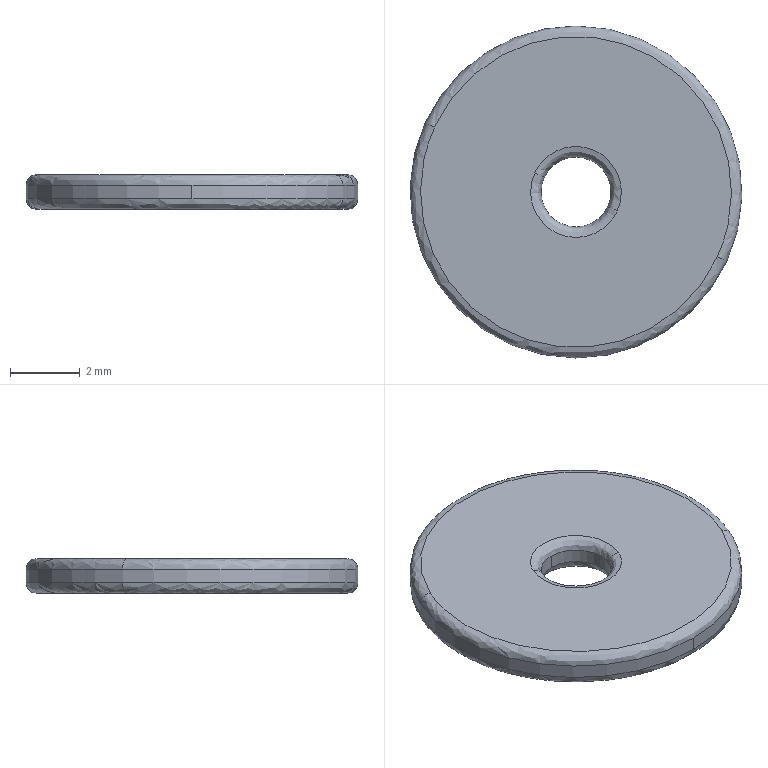Part | SolidWorks | features BaseBody 1 | 1 solid | 14 faces | box 9.5 x 9.5 x 1 mm | volume 66.343 mm3 | spline 8 | cylinder 4 | plane 2 | commonest cylinder face diameters 2 x2 9.5 x2
STEP:
#1=CARTESIAN_POINT('',(562.414,-175.786,282.579));
#2=VERTEX_POINT('',#1);
#3=CARTESIAN_POINT('',(554.328,-172.067,282.579));
#4=VERTEX_POINT('',#3);
#5=CARTESIAN_POINT('',(562.414,-175.786,282.579));
#6=CARTESIAN_POINT('',(558.694,-183.872,282.579));
#7=CARTESIAN_POINT('',(550.609,-180.152,282.579));
#8=CARTESIAN_POINT('',(554.328,-172.067,282.579));
#9=(BOUNDED_CURVE()B_SPLINE_CURVE(3,(#5,#6,#7,#8),.UNSPECIFIED.,.F.,.F.)B_SPLINE_CURVE_WITH_KNOTS((4,4),(0.,1.),.UNSPECIFIED.)CURVE()GEOMETRIC_REPRESENTATION_ITEM()RATIONAL_B_SPLINE_CURVE((1.,0.3333,0.3333,1.))REPRESENTATION_ITEM(''));
#10=EDGE_CURVE('',#2,#4,#9,.T.);
#11=ORIENTED_EDGE('',*,*,#10,.T.);
#12=CARTESIAN_POINT('',(554.056,-171.941,282.279));
#13=VERTEX_POINT('',#12);
#14=CARTESIAN_POINT('',(554.328,-172.067,282.279));
#15=DIRECTION('',(-0.4179,-0.9085,-0.000000003));
#16=DIRECTION('',(-0.9085,0.4179,0.000000002));
#17=AXIS2_PLACEMENT_3D('',#14,#15,#16);
#18=CIRCLE('',#17,0.3);
#19=EDGE_CURVE('',#4,#13,#18,.T.);
#20=ORIENTED_EDGE('',*,*,#19,.T.);
#21=CARTESIAN_POINT('',(558.371,-178.677,282.279));
#22=VERTEX_POINT('',#21);
#23=CARTESIAN_POINT('',(558.371,-173.927,282.279));
#24=DIRECTION('',(0.000000001,-0.000000003,1.));
#25=DIRECTION('',(0.9085,-0.4179,-0.000000002));
#26=AXIS2_PLACEMENT_3D('',#23,#24,#25);
#27=CIRCLE('',#26,4.75);
#28=EDGE_CURVE('',#13,#22,#27,.T.);
#29=ORIENTED_EDGE('',*,*,#28,.T.);
#30=CARTESIAN_POINT('',(562.686,-175.912,282.279));
#31=VERTEX_POINT('',#30);
#32=CARTESIAN_POINT('',(558.371,-173.927,282.279));
#33=DIRECTION('',(0.000000001,-0.000000003,1.));
#34=DIRECTION('',(0.9085,-0.4179,-0.000000002));
#35=AXIS2_PLACEMENT_3D('',#32,#33,#34);
#36=CIRCLE('',#35,4.75);
#37=EDGE_CURVE('',#22,#31,#36,.T.);
#38=ORIENTED_EDGE('',*,*,#37,.T.);
#39=CARTESIAN_POINT('',(562.414,-175.786,282.279));
#40=DIRECTION('',(0.4179,0.9085,0.000000003));
#41=DIRECTION('',(0.9085,-0.4179,-0.000000002));
#42=AXIS2_PLACEMENT_3D('',#39,#40,#41);
#43=CIRCLE('',#42,0.3);
#44=EDGE_CURVE('',#2,#31,#43,.T.);
#45=ORIENTED_EDGE('',*,*,#44,.F.);
#46=EDGE_LOOP('',(#11,#20,#29,#38,#45));
#47=FACE_OUTER_BOUND('',#46,.T.);
#48=CARTESIAN_POINT('',(554.328,-172.067,282.579));
#49=CARTESIAN_POINT('',(550.609,-180.152,282.579));
#50=CARTESIAN_POINT('',(558.694,-183.872,282.579));
#51=CARTESIAN_POINT('',(562.414,-175.786,282.579));
#52=CARTESIAN_POINT('',(554.169,-171.993,282.579));
#53=CARTESIAN_POINT('',(550.302,-180.398,282.579));
#54=CARTESIAN_POINT('',(558.707,-184.265,282.579));
#55=CARTESIAN_POINT('',(562.573,-175.86,282.579));
#56=CARTESIAN_POINT('',(554.056,-171.941,282.455));
#57=CARTESIAN_POINT('',(550.085,-180.572,282.455));
#58=CARTESIAN_POINT('',(558.716,-184.542,282.455));
#59=CARTESIAN_POINT('',(562.686,-175.912,282.455));
#60=CARTESIAN_POINT('',(554.056,-171.941,282.279));
#61=CARTESIAN_POINT('',(550.085,-180.572,282.279));
#62=CARTESIAN_POINT('',(558.716,-184.542,282.279));
#63=CARTESIAN_POINT('',(562.686,-175.912,282.279));
#64=(BOUNDED_SURFACE()B_SPLINE_SURFACE(3,3,((#48,#49,#50,#51),(#52,#53,#54,#55),(#56,#57,#58,#59),(#60,#61,#62,#63)),.UNSPECIFIED.,.F.,.F.,.T.)B_SPLINE_SURFACE_WITH_KNOTS((4,4),(4,4),(0.,1.),(0.,1.),.UNSPECIFIED.)GEOMETRIC_REPRESENTATION_ITEM()RATIONAL_B_SPLINE_SURFACE(((1.,0.3333,0.3333,1.),(0.8047,0.2682,0.2682,0.8047),(0.8047,0.2682,0.2682,0.8047),(1.,0.3333,0.3333,1.)))REPRESENTATION_ITEM('')SURFACE());
#65=ADVANCED_FACE('',(#47),#64,.T.);
#66=CARTESIAN_POINT('',(558.371,-174.927,282.279));
#67=VERTEX_POINT('',#66);
#68=CARTESIAN_POINT('',(557.463,-173.509,282.279));
#69=VERTEX_POINT('',#68);
#70=CARTESIAN_POINT('',(558.371,-173.927,282.279));
#71=DIRECTION('',(-0.000000001,0.000000003,-1.));
#72=DIRECTION('',(0.9085,-0.4179,-0.000000002));
#73=AXIS2_PLACEMENT_3D('',#70,#71,#72);
#74=CIRCLE('',#73,1.);
#75=EDGE_CURVE('',#67,#69,#74,.T.);
#76=ORIENTED_EDGE('',*,*,#75,.T.);
#77=CARTESIAN_POINT('',(557.19,-173.383,282.579));
#78=VERTEX_POINT('',#77);
#79=CARTESIAN_POINT('',(557.19,-173.383,282.279));
#80=DIRECTION('',(-0.4179,-0.9085,-0.000000003));
#81=DIRECTION('',(-0.9085,0.4179,0.000000002));
#82=AXIS2_PLACEMENT_3D('',#79,#80,#81);
#83=CIRCLE('',#82,0.3);
#84=EDGE_CURVE('',#69,#78,#83,.T.);
#85=ORIENTED_EDGE('',*,*,#84,.T.);
#86=CARTESIAN_POINT('',(559.552,-174.47,282.579));
#87=VERTEX_POINT('',#86);
#88=CARTESIAN_POINT('',(557.19,-173.383,282.579));
#89=CARTESIAN_POINT('',(556.103,-175.745,282.579));
#90=CARTESIAN_POINT('',(558.465,-176.832,282.579));
#91=CARTESIAN_POINT('',(559.552,-174.47,282.579));
#92=(BOUNDED_CURVE()B_SPLINE_CURVE(3,(#88,#89,#90,#91),.UNSPECIFIED.,.F.,.T.)B_SPLINE_CURVE_WITH_KNOTS((4,4),(0.,1.),.UNSPECIFIED.)CURVE()GEOMETRIC_REPRESENTATION_ITEM()RATIONAL_B_SPLINE_CURVE((1.,0.3333,0.3333,1.))REPRESENTATION_ITEM(''));
#93=EDGE_CURVE('',#78,#87,#92,.T.);
#94=ORIENTED_EDGE('',*,*,#93,.T.);
#95=CARTESIAN_POINT('',(559.279,-174.345,282.279));
#96=VERTEX_POINT('',#95);
#97=CARTESIAN_POINT('',(559.552,-174.47,282.279));
#98=DIRECTION('',(0.4179,0.9085,0.000000003));
#99=DIRECTION('',(0.9085,-0.4179,-0.000000002));
#100=AXIS2_PLACEMENT_3D('',#97,#98,#99);
#101=CIRCLE('',#100,0.3);
#102=EDGE_CURVE('',#96,#87,#101,.T.);
#103=ORIENTED_EDGE('',*,*,#102,.F.);
#104=CARTESIAN_POINT('',(558.371,-173.927,282.279));
#105=DIRECTION('',(-0.000000001,0.000000003,-1.));
#106=DIRECTION('',(0.9085,-0.4179,-0.000000002));
#107=AXIS2_PLACEMENT_3D('',#104,#105,#106);
#108=CIRCLE('',#107,1.);
#109=EDGE_CURVE('',#96,#67,#108,.T.);
#110=ORIENTED_EDGE('',*,*,#109,.T.);
#111=EDGE_LOOP('',(#76,#85,#94,#103,#110));
#112=FACE_OUTER_BOUND('',#111,.T.);
#113=CARTESIAN_POINT('',(557.463,-173.509,282.279));
#114=CARTESIAN_POINT('',(556.627,-175.326,282.279));
#115=CARTESIAN_POINT('',(558.444,-176.161,282.279));
#116=CARTESIAN_POINT('',(559.279,-174.345,282.279));
#117=CARTESIAN_POINT('',(557.463,-173.509,282.455));
#118=CARTESIAN_POINT('',(556.627,-175.326,282.455));
#119=CARTESIAN_POINT('',(558.444,-176.161,282.455));
#120=CARTESIAN_POINT('',(559.279,-174.345,282.455));
#121=CARTESIAN_POINT('',(557.35,-173.457,282.579));
#122=CARTESIAN_POINT('',(556.41,-175.499,282.579));
#123=CARTESIAN_POINT('',(558.453,-176.439,282.579));
#124=CARTESIAN_POINT('',(559.392,-174.396,282.579));
#125=CARTESIAN_POINT('',(557.19,-173.383,282.579));
#126=CARTESIAN_POINT('',(556.103,-175.745,282.579));
#127=CARTESIAN_POINT('',(558.465,-176.832,282.579));
#128=CARTESIAN_POINT('',(559.552,-174.47,282.579));
#129=(BOUNDED_SURFACE()B_SPLINE_SURFACE(3,3,((#113,#114,#115,#116),(#117,#118,#119,#120),(#121,#122,#123,#124),(#125,#126,#127,#128)),.UNSPECIFIED.,.F.,.F.,.T.)B_SPLINE_SURFACE_WITH_KNOTS((4,4),(4,4),(0.,1.),(0.,1.),.UNSPECIFIED.)GEOMETRIC_REPRESENTATION_ITEM()RATIONAL_B_SPLINE_SURFACE(((1.,0.3333,0.3333,1.),(0.8047,0.2682,0.2682,0.8047),(0.8047,0.2682,0.2682,0.8047),(1.,0.3333,0.3333,1.)))REPRESENTATION_ITEM('')SURFACE());
#130=ADVANCED_FACE('',(#112),#129,.T.);
#131=CARTESIAN_POINT('',(562.414,-175.786,281.579));
#132=VERTEX_POINT('',#131);
#133=CARTESIAN_POINT('',(554.328,-172.067,281.579));
#134=VERTEX_POINT('',#133);
#135=CARTESIAN_POINT('',(562.414,-175.786,281.579));
#136=CARTESIAN_POINT('',(566.133,-167.701,281.579));
#137=CARTESIAN_POINT('',(558.048,-163.981,281.579));
#138=CARTESIAN_POINT('',(554.328,-172.067,281.579));
#139=(BOUNDED_CURVE()B_SPLINE_CURVE(3,(#135,#136,#137,#138),.UNSPECIFIED.,.F.,.T.)B_SPLINE_CURVE_WITH_KNOTS((4,4),(0.,1.),.UNSPECIFIED.)CURVE()GEOMETRIC_REPRESENTATION_ITEM()RATIONAL_B_SPLINE_CURVE((1.,0.3333,0.3333,1.))REPRESENTATION_ITEM(''));
#140=EDGE_CURVE('',#132,#134,#139,.T.);
#141=ORIENTED_EDGE('',*,*,#140,.T.);
#142=CARTESIAN_POINT('',(554.056,-171.941,281.879));
#143=VERTEX_POINT('',#142);
#144=CARTESIAN_POINT('',(554.328,-172.067,281.879));
#145=DIRECTION('',(0.4179,0.9085,0.000000003));
#146=DIRECTION('',(-0.9085,0.4179,0.000000002));
#147=AXIS2_PLACEMENT_3D('',#144,#145,#146);
#148=CIRCLE('',#147,0.3);
#149=EDGE_CURVE('',#134,#143,#148,.T.);
#150=ORIENTED_EDGE('',*,*,#149,.T.);
#151=CARTESIAN_POINT('',(558.371,-169.177,281.879));
#152=VERTEX_POINT('',#151);
#153=CARTESIAN_POINT('',(558.371,-173.927,281.879));
#154=DIRECTION('',(0.000000001,-0.000000003,1.));
#155=DIRECTION('',(0.,-1.,-0.000000003));
#156=AXIS2_PLACEMENT_3D('',#153,#154,#155);
#157=CIRCLE('',#156,4.75);
#158=EDGE_CURVE('',#152,#143,#157,.T.);
#159=ORIENTED_EDGE('',*,*,#158,.F.);
#160=CARTESIAN_POINT('',(562.686,-175.912,281.879));
#161=VERTEX_POINT('',#160);
#162=CARTESIAN_POINT('',(558.371,-173.927,281.879));
#163=DIRECTION('',(0.000000001,-0.000000003,1.));
#164=DIRECTION('',(0.,-1.,-0.000000003));
#165=AXIS2_PLACEMENT_3D('',#162,#163,#164);
#166=CIRCLE('',#165,4.75);
#167=EDGE_CURVE('',#161,#152,#166,.T.);
#168=ORIENTED_EDGE('',*,*,#167,.F.);
#169=CARTESIAN_POINT('',(562.414,-175.786,281.879));
#170=DIRECTION('',(-0.4179,-0.9085,-0.000000003));
#171=DIRECTION('',(0.9085,-0.4179,-0.000000002));
#172=AXIS2_PLACEMENT_3D('',#169,#170,#171);
#173=CIRCLE('',#172,0.3);
#174=EDGE_CURVE('',#132,#161,#173,.T.);
#175=ORIENTED_EDGE('',*,*,#174,.F.);
#176=EDGE_LOOP('',(#141,#150,#159,#168,#175));
#177=FACE_OUTER_BOUND('',#176,.T.);
#178=CARTESIAN_POINT('',(554.328,-172.067,281.579));
#179=CARTESIAN_POINT('',(558.048,-163.981,281.579));
#180=CARTESIAN_POINT('',(566.133,-167.701,281.579));
#181=CARTESIAN_POINT('',(562.414,-175.786,281.579));
#182=CARTESIAN_POINT('',(554.169,-171.993,281.579));
#183=CARTESIAN_POINT('',(558.035,-163.589,281.579));
#184=CARTESIAN_POINT('',(566.44,-167.455,281.579));
#185=CARTESIAN_POINT('',(562.573,-175.86,281.579));
#186=CARTESIAN_POINT('',(554.056,-171.941,281.703));
#187=CARTESIAN_POINT('',(558.026,-163.311,281.703));
#188=CARTESIAN_POINT('',(566.657,-167.281,281.703));
#189=CARTESIAN_POINT('',(562.686,-175.912,281.703));
#190=CARTESIAN_POINT('',(554.056,-171.941,281.879));
#191=CARTESIAN_POINT('',(558.026,-163.311,281.879));
#192=CARTESIAN_POINT('',(566.657,-167.281,281.879));
#193=CARTESIAN_POINT('',(562.686,-175.912,281.879));
#194=(BOUNDED_SURFACE()B_SPLINE_SURFACE(3,3,((#178,#179,#180,#181),(#182,#183,#184,#185),(#186,#187,#188,#189),(#190,#191,#192,#193)),.UNSPECIFIED.,.F.,.F.,.T.)B_SPLINE_SURFACE_WITH_KNOTS((4,4),(4,4),(0.,1.),(0.,1.),.UNSPECIFIED.)GEOMETRIC_REPRESENTATION_ITEM()RATIONAL_B_SPLINE_SURFACE(((1.,0.3333,0.3333,1.),(0.8047,0.2682,0.2682,0.8047),(0.8047,0.2682,0.2682,0.8047),(1.,0.3333,0.3333,1.)))REPRESENTATION_ITEM('')SURFACE());
#195=ADVANCED_FACE('',(#177),#194,.T.);
#196=CARTESIAN_POINT('',(558.371,-172.927,281.879));
#197=VERTEX_POINT('',#196);
#198=CARTESIAN_POINT('',(557.463,-173.509,281.879));
#199=VERTEX_POINT('',#198);
#200=CARTESIAN_POINT('',(558.371,-173.927,281.879));
#201=DIRECTION('',(0.000000001,-0.000000003,1.));
#202=DIRECTION('',(0.,1.,0.000000003));
#203=AXIS2_PLACEMENT_3D('',#200,#201,#202);
#204=CIRCLE('',#203,1.);
#205=EDGE_CURVE('',#197,#199,#204,.T.);
#206=ORIENTED_EDGE('',*,*,#205,.T.);
#207=CARTESIAN_POINT('',(557.19,-173.383,281.579));
#208=VERTEX_POINT('',#207);
#209=CARTESIAN_POINT('',(557.19,-173.383,281.879));
#210=DIRECTION('',(0.4179,0.9085,0.000000003));
#211=DIRECTION('',(-0.9085,0.4179,0.000000002));
#212=AXIS2_PLACEMENT_3D('',#209,#210,#211);
#213=CIRCLE('',#212,0.3);
#214=EDGE_CURVE('',#199,#208,#213,.T.);
#215=ORIENTED_EDGE('',*,*,#214,.T.);
#216=CARTESIAN_POINT('',(559.552,-174.47,281.579));
#217=VERTEX_POINT('',#216);
#218=CARTESIAN_POINT('',(557.19,-173.383,281.579));
#219=CARTESIAN_POINT('',(558.277,-171.021,281.579));
#220=CARTESIAN_POINT('',(560.639,-172.108,281.579));
#221=CARTESIAN_POINT('',(559.552,-174.47,281.579));
#222=(BOUNDED_CURVE()B_SPLINE_CURVE(3,(#218,#219,#220,#221),.UNSPECIFIED.,.F.,.F.)B_SPLINE_CURVE_WITH_KNOTS((4,4),(0.,1.),.UNSPECIFIED.)CURVE()GEOMETRIC_REPRESENTATION_ITEM()RATIONAL_B_SPLINE_CURVE((1.,0.3333,0.3333,1.))REPRESENTATION_ITEM(''));
#223=EDGE_CURVE('',#208,#217,#222,.T.);
#224=ORIENTED_EDGE('',*,*,#223,.T.);
#225=CARTESIAN_POINT('',(559.279,-174.345,281.879));
#226=VERTEX_POINT('',#225);
#227=CARTESIAN_POINT('',(559.552,-174.47,281.879));
#228=DIRECTION('',(-0.4179,-0.9085,-0.000000003));
#229=DIRECTION('',(0.9085,-0.4179,-0.000000002));
#230=AXIS2_PLACEMENT_3D('',#227,#228,#229);
#231=CIRCLE('',#230,0.3);
#232=EDGE_CURVE('',#226,#217,#231,.T.);
#233=ORIENTED_EDGE('',*,*,#232,.F.);
#234=CARTESIAN_POINT('',(558.371,-173.927,281.879));
#235=DIRECTION('',(0.000000001,-0.000000003,1.));
#236=DIRECTION('',(0.,1.,0.000000003));
#237=AXIS2_PLACEMENT_3D('',#234,#235,#236);
#238=CIRCLE('',#237,1.);
#239=EDGE_CURVE('',#226,#197,#238,.T.);
#240=ORIENTED_EDGE('',*,*,#239,.T.);
#241=EDGE_LOOP('',(#206,#215,#224,#233,#240));
#242=FACE_OUTER_BOUND('',#241,.T.);
#243=CARTESIAN_POINT('',(557.463,-173.509,281.879));
#244=CARTESIAN_POINT('',(558.298,-171.692,281.879));
#245=CARTESIAN_POINT('',(560.115,-172.528,281.879));
#246=CARTESIAN_POINT('',(559.279,-174.345,281.879));
#247=CARTESIAN_POINT('',(557.463,-173.509,281.703));
#248=CARTESIAN_POINT('',(558.298,-171.692,281.703));
#249=CARTESIAN_POINT('',(560.115,-172.528,281.703));
#250=CARTESIAN_POINT('',(559.279,-174.345,281.703));
#251=CARTESIAN_POINT('',(557.35,-173.457,281.579));
#252=CARTESIAN_POINT('',(558.289,-171.414,281.579));
#253=CARTESIAN_POINT('',(560.332,-172.354,281.579));
#254=CARTESIAN_POINT('',(559.392,-174.396,281.579));
#255=CARTESIAN_POINT('',(557.19,-173.383,281.579));
#256=CARTESIAN_POINT('',(558.277,-171.021,281.579));
#257=CARTESIAN_POINT('',(560.639,-172.108,281.579));
#258=CARTESIAN_POINT('',(559.552,-174.47,281.579));
#259=(BOUNDED_SURFACE()B_SPLINE_SURFACE(3,3,((#243,#244,#245,#246),(#247,#248,#249,#250),(#251,#252,#253,#254),(#255,#256,#257,#258)),.UNSPECIFIED.,.F.,.F.,.F.)B_SPLINE_SURFACE_WITH_KNOTS((4,4),(4,4),(0.,1.),(0.,1.),.UNSPECIFIED.)GEOMETRIC_REPRESENTATION_ITEM()RATIONAL_B_SPLINE_SURFACE(((1.,0.3333,0.3333,1.),(0.8047,0.2682,0.2682,0.8047),(0.8047,0.2682,0.2682,0.8047),(1.,0.3333,0.3333,1.)))REPRESENTATION_ITEM('')SURFACE());
#260=ADVANCED_FACE('',(#242),#259,.T.);
#261=CARTESIAN_POINT('',(558.371,-178.677,281.879));
#262=VERTEX_POINT('',#261);
#263=CARTESIAN_POINT('',(558.371,-173.927,281.879));
#264=DIRECTION('',(0.000000001,-0.000000003,1.));
#265=DIRECTION('',(0.,-1.,-0.000000003));
#266=AXIS2_PLACEMENT_3D('',#263,#264,#265);
#267=CIRCLE('',#266,4.75);
#268=EDGE_CURVE('',#262,#161,#267,.T.);
#269=ORIENTED_EDGE('',*,*,#268,.T.);
#270=ORIENTED_EDGE('',*,*,#167,.T.);
#271=CARTESIAN_POINT('',(558.371,-169.177,282.279));
#272=VERTEX_POINT('',#271);
#273=CARTESIAN_POINT('',(558.371,-169.177,282.579));
#274=DIRECTION('',(0.000000001,-0.000000003,1.));
#275=VECTOR('',#274,1000.);
#276=LINE('',#273,#275);
#277=EDGE_CURVE('',#152,#272,#276,.T.);
#278=ORIENTED_EDGE('',*,*,#277,.T.);
#279=CARTESIAN_POINT('',(558.371,-173.927,282.279));
#280=DIRECTION('',(0.000000001,-0.000000003,1.));
#281=DIRECTION('',(0.9085,-0.4179,-0.000000002));
#282=AXIS2_PLACEMENT_3D('',#279,#280,#281);
#283=CIRCLE('',#282,4.75);
#284=EDGE_CURVE('',#31,#272,#283,.T.);
#285=ORIENTED_EDGE('',*,*,#284,.F.);
#286=ORIENTED_EDGE('',*,*,#37,.F.);
#287=CARTESIAN_POINT('',(558.371,-178.677,282.579));
#288=DIRECTION('',(0.000000001,-0.000000003,1.));
#289=VECTOR('',#288,1000.);
#290=LINE('',#287,#289);
#291=EDGE_CURVE('',#262,#22,#290,.T.);
#292=ORIENTED_EDGE('',*,*,#291,.F.);
#293=EDGE_LOOP('',(#269,#270,#278,#285,#286,#292));
#294=FACE_OUTER_BOUND('',#293,.T.);
#295=CARTESIAN_POINT('',(558.371,-173.927,282.579));
#296=DIRECTION('',(0.000000001,-0.000000003,1.));
#297=DIRECTION('',(0.,-1.,-0.000000003));
#298=AXIS2_PLACEMENT_3D('',#295,#296,#297);
#299=CYLINDRICAL_SURFACE('',#298,4.75);
#300=ADVANCED_FACE('',(#294),#299,.T.);
#301=ORIENTED_EDGE('',*,*,#75,.F.);
#302=CARTESIAN_POINT('',(558.371,-174.927,281.879));
#303=VERTEX_POINT('',#302);
#304=CARTESIAN_POINT('',(558.371,-174.927,281.579));
#305=DIRECTION('',(-0.000000001,0.000000003,-1.));
#306=VECTOR('',#305,1000.);
#307=LINE('',#304,#306);
#308=EDGE_CURVE('',#67,#303,#307,.T.);
#309=ORIENTED_EDGE('',*,*,#308,.T.);
#310=CARTESIAN_POINT('',(558.371,-173.927,281.879));
#311=DIRECTION('',(0.000000001,-0.000000003,1.));
#312=DIRECTION('',(0.,1.,0.000000003));
#313=AXIS2_PLACEMENT_3D('',#310,#311,#312);
#314=CIRCLE('',#313,1.);
#315=EDGE_CURVE('',#199,#303,#314,.T.);
#316=ORIENTED_EDGE('',*,*,#315,.F.);
#317=ORIENTED_EDGE('',*,*,#205,.F.);
#318=CARTESIAN_POINT('',(558.371,-172.927,282.279));
#319=VERTEX_POINT('',#318);
#320=CARTESIAN_POINT('',(558.371,-172.927,281.579));
#321=DIRECTION('',(-0.000000001,0.000000003,-1.));
#322=VECTOR('',#321,1000.);
#323=LINE('',#320,#322);
#324=EDGE_CURVE('',#319,#197,#323,.T.);
#325=ORIENTED_EDGE('',*,*,#324,.F.);
#326=CARTESIAN_POINT('',(558.371,-173.927,282.279));
#327=DIRECTION('',(-0.000000001,0.000000003,-1.));
#328=DIRECTION('',(0.9085,-0.4179,-0.000000002));
#329=AXIS2_PLACEMENT_3D('',#326,#327,#328);
#330=CIRCLE('',#329,1.);
#331=EDGE_CURVE('',#69,#319,#330,.T.);
#332=ORIENTED_EDGE('',*,*,#331,.F.);
#333=EDGE_LOOP('',(#301,#309,#316,#317,#325,#332));
#334=FACE_OUTER_BOUND('',#333,.T.);
#335=CARTESIAN_POINT('',(558.371,-173.927,281.579));
#336=DIRECTION('',(-0.000000001,0.000000003,-1.));
#337=DIRECTION('',(0.,1.,0.000000003));
#338=AXIS2_PLACEMENT_3D('',#335,#336,#337);
#339=CYLINDRICAL_SURFACE('',#338,1.);
#340=ADVANCED_FACE('',(#334),#339,.F.);
#341=ORIENTED_EDGE('',*,*,#10,.F.);
#342=CARTESIAN_POINT('',(554.328,-172.067,282.579));
#343=CARTESIAN_POINT('',(558.048,-163.981,282.579));
#344=CARTESIAN_POINT('',(566.133,-167.701,282.579));
#345=CARTESIAN_POINT('',(562.414,-175.786,282.579));
#346=(BOUNDED_CURVE()B_SPLINE_CURVE(3,(#342,#343,#344,#345),.UNSPECIFIED.,.F.,.F.)B_SPLINE_CURVE_WITH_KNOTS((4,4),(0.,1.),.UNSPECIFIED.)CURVE()GEOMETRIC_REPRESENTATION_ITEM()RATIONAL_B_SPLINE_CURVE((1.,0.3333,0.3333,1.))REPRESENTATION_ITEM(''));
#347=EDGE_CURVE('',#4,#2,#346,.T.);
#348=ORIENTED_EDGE('',*,*,#347,.F.);
#349=EDGE_LOOP('',(#341,#348));
#350=FACE_OUTER_BOUND('',#349,.T.);
#351=CARTESIAN_POINT('',(559.552,-174.47,282.579));
#352=CARTESIAN_POINT('',(560.639,-172.108,282.579));
#353=CARTESIAN_POINT('',(558.277,-171.021,282.579));
#354=CARTESIAN_POINT('',(557.19,-173.383,282.579));
#355=(BOUNDED_CURVE()B_SPLINE_CURVE(3,(#351,#352,#353,#354),.UNSPECIFIED.,.F.,.T.)B_SPLINE_CURVE_WITH_KNOTS((4,4),(0.,1.),.UNSPECIFIED.)CURVE()GEOMETRIC_REPRESENTATION_ITEM()RATIONAL_B_SPLINE_CURVE((1.,0.3333,0.3333,1.))REPRESENTATION_ITEM(''));
#356=EDGE_CURVE('',#87,#78,#355,.T.);
#357=ORIENTED_EDGE('',*,*,#356,.F.);
#358=ORIENTED_EDGE('',*,*,#93,.F.);
#359=EDGE_LOOP('',(#357,#358));
#360=FACE_BOUND('',#359,.T.);
#361=CARTESIAN_POINT('',(558.371,-173.927,282.579));
#362=DIRECTION('',(-0.000000001,0.000000003,-1.));
#363=DIRECTION('',(0.,1.,0.000000003));
#364=AXIS2_PLACEMENT_3D('',#361,#362,#363);
#365=PLANE('',#364);
#366=ADVANCED_FACE('',(#350,#360),#365,.F.);
#367=ORIENTED_EDGE('',*,*,#19,.F.);
#368=ORIENTED_EDGE('',*,*,#347,.T.);
#369=ORIENTED_EDGE('',*,*,#44,.T.);
#370=ORIENTED_EDGE('',*,*,#284,.T.);
#371=CARTESIAN_POINT('',(558.371,-173.927,282.279));
#372=DIRECTION('',(0.000000001,-0.000000003,1.));
#373=DIRECTION('',(0.9085,-0.4179,-0.000000002));
#374=AXIS2_PLACEMENT_3D('',#371,#372,#373);
#375=CIRCLE('',#374,4.75);
#376=EDGE_CURVE('',#272,#13,#375,.T.);
#377=ORIENTED_EDGE('',*,*,#376,.T.);
#378=EDGE_LOOP('',(#367,#368,#369,#370,#377));
#379=FACE_OUTER_BOUND('',#378,.T.);
#380=CARTESIAN_POINT('',(562.414,-175.786,282.579));
#381=CARTESIAN_POINT('',(566.133,-167.701,282.579));
#382=CARTESIAN_POINT('',(558.048,-163.981,282.579));
#383=CARTESIAN_POINT('',(554.328,-172.067,282.579));
#384=CARTESIAN_POINT('',(562.573,-175.86,282.579));
#385=CARTESIAN_POINT('',(566.44,-167.455,282.579));
#386=CARTESIAN_POINT('',(558.035,-163.589,282.579));
#387=CARTESIAN_POINT('',(554.169,-171.993,282.579));
#388=CARTESIAN_POINT('',(562.686,-175.912,282.455));
#389=CARTESIAN_POINT('',(566.657,-167.281,282.455));
#390=CARTESIAN_POINT('',(558.026,-163.311,282.455));
#391=CARTESIAN_POINT('',(554.056,-171.941,282.455));
#392=CARTESIAN_POINT('',(562.686,-175.912,282.279));
#393=CARTESIAN_POINT('',(566.657,-167.281,282.279));
#394=CARTESIAN_POINT('',(558.026,-163.311,282.279));
#395=CARTESIAN_POINT('',(554.056,-171.941,282.279));
#396=(BOUNDED_SURFACE()B_SPLINE_SURFACE(3,3,((#380,#381,#382,#383),(#384,#385,#386,#387),(#388,#389,#390,#391),(#392,#393,#394,#395)),.UNSPECIFIED.,.F.,.F.,.F.)B_SPLINE_SURFACE_WITH_KNOTS((4,4),(4,4),(0.,1.),(0.,1.),.UNSPECIFIED.)GEOMETRIC_REPRESENTATION_ITEM()RATIONAL_B_SPLINE_SURFACE(((1.,0.3333,0.3333,1.),(0.8047,0.2682,0.2682,0.8047),(0.8047,0.2682,0.2682,0.8047),(1.,0.3333,0.3333,1.)))REPRESENTATION_ITEM('')SURFACE());
#397=ADVANCED_FACE('',(#379),#396,.T.);
#398=ORIENTED_EDGE('',*,*,#84,.F.);
#399=ORIENTED_EDGE('',*,*,#331,.T.);
#400=CARTESIAN_POINT('',(558.371,-173.927,282.279));
#401=DIRECTION('',(-0.000000001,0.000000003,-1.));
#402=DIRECTION('',(0.9085,-0.4179,-0.000000002));
#403=AXIS2_PLACEMENT_3D('',#400,#401,#402);
#404=CIRCLE('',#403,1.);
#405=EDGE_CURVE('',#319,#96,#404,.T.);
#406=ORIENTED_EDGE('',*,*,#405,.T.);
#407=ORIENTED_EDGE('',*,*,#102,.T.);
#408=ORIENTED_EDGE('',*,*,#356,.T.);
#409=EDGE_LOOP('',(#398,#399,#406,#407,#408));
#410=FACE_OUTER_BOUND('',#409,.T.);
#411=CARTESIAN_POINT('',(559.279,-174.345,282.279));
#412=CARTESIAN_POINT('',(560.115,-172.528,282.279));
#413=CARTESIAN_POINT('',(558.298,-171.692,282.279));
#414=CARTESIAN_POINT('',(557.463,-173.509,282.279));
#415=CARTESIAN_POINT('',(559.279,-174.345,282.455));
#416=CARTESIAN_POINT('',(560.115,-172.528,282.455));
#417=CARTESIAN_POINT('',(558.298,-171.692,282.455));
#418=CARTESIAN_POINT('',(557.463,-173.509,282.455));
#419=CARTESIAN_POINT('',(559.392,-174.396,282.579));
#420=CARTESIAN_POINT('',(560.332,-172.354,282.579));
#421=CARTESIAN_POINT('',(558.289,-171.414,282.579));
#422=CARTESIAN_POINT('',(557.35,-173.457,282.579));
#423=CARTESIAN_POINT('',(559.552,-174.47,282.579));
#424=CARTESIAN_POINT('',(560.639,-172.108,282.579));
#425=CARTESIAN_POINT('',(558.277,-171.021,282.579));
#426=CARTESIAN_POINT('',(557.19,-173.383,282.579));
#427=(BOUNDED_SURFACE()B_SPLINE_SURFACE(3,3,((#411,#412,#413,#414),(#415,#416,#417,#418),(#419,#420,#421,#422),(#423,#424,#425,#426)),.UNSPECIFIED.,.F.,.F.,.T.)B_SPLINE_SURFACE_WITH_KNOTS((4,4),(4,4),(0.,1.),(0.,1.),.UNSPECIFIED.)GEOMETRIC_REPRESENTATION_ITEM()RATIONAL_B_SPLINE_SURFACE(((1.,0.3333,0.3333,1.),(0.8047,0.2682,0.2682,0.8047),(0.8047,0.2682,0.2682,0.8047),(1.,0.3333,0.3333,1.)))REPRESENTATION_ITEM('')SURFACE());
#428=ADVANCED_FACE('',(#410),#427,.T.);
#429=ORIENTED_EDGE('',*,*,#277,.F.);
#430=ORIENTED_EDGE('',*,*,#158,.T.);
#431=CARTESIAN_POINT('',(558.371,-173.927,281.879));
#432=DIRECTION('',(0.000000001,-0.000000003,1.));
#433=DIRECTION('',(0.,-1.,-0.000000003));
#434=AXIS2_PLACEMENT_3D('',#431,#432,#433);
#435=CIRCLE('',#434,4.75);
#436=EDGE_CURVE('',#143,#262,#435,.T.);
#437=ORIENTED_EDGE('',*,*,#436,.T.);
#438=ORIENTED_EDGE('',*,*,#291,.T.);
#439=ORIENTED_EDGE('',*,*,#28,.F.);
#440=ORIENTED_EDGE('',*,*,#376,.F.);
#441=EDGE_LOOP('',(#429,#430,#437,#438,#439,#440));
#442=FACE_OUTER_BOUND('',#441,.T.);
#443=CARTESIAN_POINT('',(558.371,-173.927,282.579));
#444=DIRECTION('',(0.000000001,-0.000000003,1.));
#445=DIRECTION('',(0.,-1.,-0.000000003));
#446=AXIS2_PLACEMENT_3D('',#443,#444,#445);
#447=CYLINDRICAL_SURFACE('',#446,4.75);
#448=ADVANCED_FACE('',(#442),#447,.T.);
#449=ORIENTED_EDGE('',*,*,#308,.F.);
#450=ORIENTED_EDGE('',*,*,#109,.F.);
#451=ORIENTED_EDGE('',*,*,#405,.F.);
#452=ORIENTED_EDGE('',*,*,#324,.T.);
#453=ORIENTED_EDGE('',*,*,#239,.F.);
#454=CARTESIAN_POINT('',(558.371,-173.927,281.879));
#455=DIRECTION('',(0.000000001,-0.000000003,1.));
#456=DIRECTION('',(0.,1.,0.000000003));
#457=AXIS2_PLACEMENT_3D('',#454,#455,#456);
#458=CIRCLE('',#457,1.);
#459=EDGE_CURVE('',#303,#226,#458,.T.);
#460=ORIENTED_EDGE('',*,*,#459,.F.);
#461=EDGE_LOOP('',(#449,#450,#451,#452,#453,#460));
#462=FACE_OUTER_BOUND('',#461,.T.);
#463=CARTESIAN_POINT('',(558.371,-173.927,281.579));
#464=DIRECTION('',(-0.000000001,0.000000003,-1.));
#465=DIRECTION('',(0.,1.,0.000000003));
#466=AXIS2_PLACEMENT_3D('',#463,#464,#465);
#467=CYLINDRICAL_SURFACE('',#466,1.);
#468=ADVANCED_FACE('',(#462),#467,.F.);
#469=ORIENTED_EDGE('',*,*,#149,.F.);
#470=CARTESIAN_POINT('',(554.328,-172.067,281.579));
#471=CARTESIAN_POINT('',(550.609,-180.152,281.579));
#472=CARTESIAN_POINT('',(558.694,-183.872,281.579));
#473=CARTESIAN_POINT('',(562.414,-175.786,281.579));
#474=(BOUNDED_CURVE()B_SPLINE_CURVE(3,(#470,#471,#472,#473),.UNSPECIFIED.,.F.,.T.)B_SPLINE_CURVE_WITH_KNOTS((4,4),(0.,1.),.UNSPECIFIED.)CURVE()GEOMETRIC_REPRESENTATION_ITEM()RATIONAL_B_SPLINE_CURVE((1.,0.3333,0.3333,1.))REPRESENTATION_ITEM(''));
#475=EDGE_CURVE('',#134,#132,#474,.T.);
#476=ORIENTED_EDGE('',*,*,#475,.T.);
#477=ORIENTED_EDGE('',*,*,#174,.T.);
#478=ORIENTED_EDGE('',*,*,#268,.F.);
#479=ORIENTED_EDGE('',*,*,#436,.F.);
#480=EDGE_LOOP('',(#469,#476,#477,#478,#479));
#481=FACE_OUTER_BOUND('',#480,.T.);
#482=CARTESIAN_POINT('',(562.414,-175.786,281.579));
#483=CARTESIAN_POINT('',(558.694,-183.872,281.579));
#484=CARTESIAN_POINT('',(550.609,-180.152,281.579));
#485=CARTESIAN_POINT('',(554.328,-172.067,281.579));
#486=CARTESIAN_POINT('',(562.573,-175.86,281.579));
#487=CARTESIAN_POINT('',(558.707,-184.265,281.579));
#488=CARTESIAN_POINT('',(550.302,-180.398,281.579));
#489=CARTESIAN_POINT('',(554.169,-171.993,281.579));
#490=CARTESIAN_POINT('',(562.686,-175.912,281.703));
#491=CARTESIAN_POINT('',(558.716,-184.542,281.703));
#492=CARTESIAN_POINT('',(550.085,-180.572,281.703));
#493=CARTESIAN_POINT('',(554.056,-171.941,281.703));
#494=CARTESIAN_POINT('',(562.686,-175.912,281.879));
#495=CARTESIAN_POINT('',(558.716,-184.542,281.879));
#496=CARTESIAN_POINT('',(550.085,-180.572,281.879));
#497=CARTESIAN_POINT('',(554.056,-171.941,281.879));
#498=(BOUNDED_SURFACE()B_SPLINE_SURFACE(3,3,((#482,#483,#484,#485),(#486,#487,#488,#489),(#490,#491,#492,#493),(#494,#495,#496,#497)),.UNSPECIFIED.,.F.,.F.,.T.)B_SPLINE_SURFACE_WITH_KNOTS((4,4),(4,4),(0.,1.),(0.,1.),.UNSPECIFIED.)GEOMETRIC_REPRESENTATION_ITEM()RATIONAL_B_SPLINE_SURFACE(((1.,0.3333,0.3333,1.),(0.8047,0.2682,0.2682,0.8047),(0.8047,0.2682,0.2682,0.8047),(1.,0.3333,0.3333,1.)))REPRESENTATION_ITEM('')SURFACE());
#499=ADVANCED_FACE('',(#481),#498,.T.);
#500=ORIENTED_EDGE('',*,*,#214,.F.);
#501=ORIENTED_EDGE('',*,*,#315,.T.);
#502=ORIENTED_EDGE('',*,*,#459,.T.);
#503=ORIENTED_EDGE('',*,*,#232,.T.);
#504=CARTESIAN_POINT('',(559.552,-174.47,281.579));
#505=CARTESIAN_POINT('',(558.465,-176.832,281.579));
#506=CARTESIAN_POINT('',(556.103,-175.745,281.579));
#507=CARTESIAN_POINT('',(557.19,-173.383,281.579));
#508=(BOUNDED_CURVE()B_SPLINE_CURVE(3,(#504,#505,#506,#507),.UNSPECIFIED.,.F.,.F.)B_SPLINE_CURVE_WITH_KNOTS((4,4),(0.,1.),.UNSPECIFIED.)CURVE()GEOMETRIC_REPRESENTATION_ITEM()RATIONAL_B_SPLINE_CURVE((1.,0.3333,0.3333,1.))REPRESENTATION_ITEM(''));
#509=EDGE_CURVE('',#217,#208,#508,.T.);
#510=ORIENTED_EDGE('',*,*,#509,.T.);
#511=EDGE_LOOP('',(#500,#501,#502,#503,#510));
#512=FACE_OUTER_BOUND('',#511,.T.);
#513=CARTESIAN_POINT('',(559.279,-174.345,281.879));
#514=CARTESIAN_POINT('',(558.444,-176.161,281.879));
#515=CARTESIAN_POINT('',(556.627,-175.326,281.879));
#516=CARTESIAN_POINT('',(557.463,-173.509,281.879));
#517=CARTESIAN_POINT('',(559.279,-174.345,281.703));
#518=CARTESIAN_POINT('',(558.444,-176.161,281.703));
#519=CARTESIAN_POINT('',(556.627,-175.326,281.703));
#520=CARTESIAN_POINT('',(557.463,-173.509,281.703));
#521=CARTESIAN_POINT('',(559.392,-174.396,281.579));
#522=CARTESIAN_POINT('',(558.453,-176.439,281.579));
#523=CARTESIAN_POINT('',(556.41,-175.499,281.579));
#524=CARTESIAN_POINT('',(557.35,-173.457,281.579));
#525=CARTESIAN_POINT('',(559.552,-174.47,281.579));
#526=CARTESIAN_POINT('',(558.465,-176.832,281.579));
#527=CARTESIAN_POINT('',(556.103,-175.745,281.579));
#528=CARTESIAN_POINT('',(557.19,-173.383,281.579));
#529=(BOUNDED_SURFACE()B_SPLINE_SURFACE(3,3,((#513,#514,#515,#516),(#517,#518,#519,#520),(#521,#522,#523,#524),(#525,#526,#527,#528)),.UNSPECIFIED.,.F.,.F.,.F.)B_SPLINE_SURFACE_WITH_KNOTS((4,4),(4,4),(0.,1.),(0.,1.),.UNSPECIFIED.)GEOMETRIC_REPRESENTATION_ITEM()RATIONAL_B_SPLINE_SURFACE(((1.,0.3333,0.3333,1.),(0.8047,0.2682,0.2682,0.8047),(0.8047,0.2682,0.2682,0.8047),(1.,0.3333,0.3333,1.)))REPRESENTATION_ITEM('')SURFACE());
#530=ADVANCED_FACE('',(#512),#529,.T.);
#531=ORIENTED_EDGE('',*,*,#475,.F.);
#532=ORIENTED_EDGE('',*,*,#140,.F.);
#533=EDGE_LOOP('',(#531,#532));
#534=FACE_OUTER_BOUND('',#533,.T.);
#535=ORIENTED_EDGE('',*,*,#223,.F.);
#536=ORIENTED_EDGE('',*,*,#509,.F.);
#537=EDGE_LOOP('',(#535,#536));
#538=FACE_BOUND('',#537,.T.);
#539=CARTESIAN_POINT('',(558.371,-173.927,281.579));
#540=DIRECTION('',(-0.000000001,0.000000003,-1.));
#541=DIRECTION('',(0.,1.,0.000000003));
#542=AXIS2_PLACEMENT_3D('',#539,#540,#541);
#543=PLANE('',#542);
#544=ADVANCED_FACE('',(#534,#538),#543,.T.);
#545=CLOSED_SHELL('',(#65,#130,#195,#260,#300,#340,#366,#397,#428,#448,#468,#499,#530,#544));
#546=MANIFOLD_SOLID_BREP('',#545);
#547=CARTESIAN_POINT('',(0.,0.,0.));
#548=DIRECTION('',(0.,0.,1.));
#549=DIRECTION('',(1.,0.,0.));
#550=AXIS2_PLACEMENT_3D('',#547,#548,#549);
#551=(LENGTH_UNIT()NAMED_UNIT(*)SI_UNIT(.MILLI.,.METRE.));
#552=UNCERTAINTY_MEASURE_WITH_UNIT(LENGTH_MEASURE(0.00001),#551,'','');
#553=(NAMED_UNIT(*)PLANE_ANGLE_UNIT()SI_UNIT($,.RADIAN.));
#554=(NAMED_UNIT(*)SI_UNIT($,.STERADIAN.)SOLID_ANGLE_UNIT());
#555=(GEOMETRIC_REPRESENTATION_CONTEXT(3)GLOBAL_UNCERTAINTY_ASSIGNED_CONTEXT((#552))GLOBAL_UNIT_ASSIGNED_CONTEXT((#551,#553,#554))REPRESENTATION_CONTEXT('',''));
#556=ADVANCED_BREP_SHAPE_REPRESENTATION('',(#546,#550),#555);